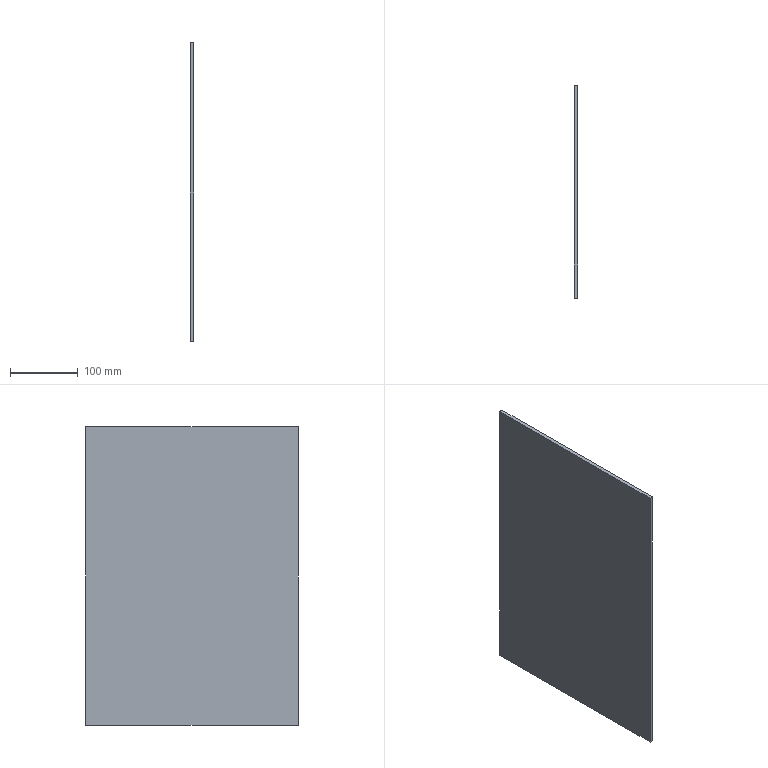Part | NX | features solid 2 | 1 solid | 6 faces | box 5 x 315 x 442 mm | volume 696150 mm3 | plane 6
STEP:
#1=CARTESIAN_POINT('',(2193.5,-894.,882.5));
#2=VERTEX_POINT('',#1);
#3=CARTESIAN_POINT('',(2193.5,-1209.,882.5));
#4=VERTEX_POINT('',#3);
#5=CARTESIAN_POINT('',(2193.5,-829.,882.5));
#6=DIRECTION('',(0.,-1.,0.));
#7=VECTOR('',#6,1000.);
#8=LINE('',#5,#7);
#9=EDGE_CURVE('',#2,#4,#8,.T.);
#10=ORIENTED_EDGE('',*,*,#9,.T.);
#11=CARTESIAN_POINT('',(2193.5,-1209.,440.5));
#12=VERTEX_POINT('',#11);
#13=CARTESIAN_POINT('',(2193.5,-1209.,972.5));
#14=DIRECTION('',(0.,0.,-1.));
#15=VECTOR('',#14,1000.);
#16=LINE('',#13,#15);
#17=EDGE_CURVE('',#4,#12,#16,.T.);
#18=ORIENTED_EDGE('',*,*,#17,.T.);
#19=CARTESIAN_POINT('',(2193.5,-894.,440.5));
#20=VERTEX_POINT('',#19);
#21=CARTESIAN_POINT('',(2193.5,-829.,440.5));
#22=DIRECTION('',(0.,1.,0.));
#23=VECTOR('',#22,1000.);
#24=LINE('',#21,#23);
#25=EDGE_CURVE('',#12,#20,#24,.T.);
#26=ORIENTED_EDGE('',*,*,#25,.T.);
#27=CARTESIAN_POINT('',(2193.5,-894.,972.5));
#28=DIRECTION('',(0.,0.,1.));
#29=VECTOR('',#28,1000.);
#30=LINE('',#27,#29);
#31=EDGE_CURVE('',#20,#2,#30,.T.);
#32=ORIENTED_EDGE('',*,*,#31,.T.);
#33=EDGE_LOOP('',(#10,#18,#26,#32));
#34=FACE_BOUND('',#33,.T.);
#35=CARTESIAN_POINT('',(2193.5,-829.,972.5));
#36=DIRECTION('',(1.,0.,0.));
#37=DIRECTION('',(0.,0.,-1.));
#38=AXIS2_PLACEMENT_3D('',#35,#36,#37);
#39=PLANE('',#38);
#40=ADVANCED_FACE('',(#34),#39,.T.);
#41=ORIENTED_EDGE('',*,*,#31,.F.);
#42=CARTESIAN_POINT('',(2188.5,-894.,440.5));
#43=VERTEX_POINT('',#42);
#44=CARTESIAN_POINT('',(2188.5,-894.,440.5));
#45=DIRECTION('',(-1.,0.,0.));
#46=VECTOR('',#45,1000.);
#47=LINE('',#44,#46);
#48=EDGE_CURVE('',#20,#43,#47,.T.);
#49=ORIENTED_EDGE('',*,*,#48,.T.);
#50=CARTESIAN_POINT('',(2188.5,-894.,882.5));
#51=VERTEX_POINT('',#50);
#52=CARTESIAN_POINT('',(2188.5,-894.,972.5));
#53=DIRECTION('',(0.,0.,1.));
#54=VECTOR('',#53,1000.);
#55=LINE('',#52,#54);
#56=EDGE_CURVE('',#43,#51,#55,.T.);
#57=ORIENTED_EDGE('',*,*,#56,.T.);
#58=CARTESIAN_POINT('',(2188.5,-894.,882.5));
#59=DIRECTION('',(-1.,0.,0.));
#60=VECTOR('',#59,1000.);
#61=LINE('',#58,#60);
#62=EDGE_CURVE('',#2,#51,#61,.T.);
#63=ORIENTED_EDGE('',*,*,#62,.F.);
#64=EDGE_LOOP('',(#41,#49,#57,#63));
#65=FACE_BOUND('',#64,.T.);
#66=CARTESIAN_POINT('',(2188.5,-894.,972.5));
#67=DIRECTION('',(0.,1.,0.));
#68=DIRECTION('',(0.,0.,-1.));
#69=AXIS2_PLACEMENT_3D('',#66,#67,#68);
#70=PLANE('',#69);
#71=ADVANCED_FACE('',(#65),#70,.T.);
#72=CARTESIAN_POINT('',(2188.5,-1209.,440.5));
#73=VERTEX_POINT('',#72);
#74=CARTESIAN_POINT('',(2188.5,-1209.,440.5));
#75=DIRECTION('',(-1.,0.,0.));
#76=VECTOR('',#75,1000.);
#77=LINE('',#74,#76);
#78=EDGE_CURVE('',#12,#73,#77,.T.);
#79=ORIENTED_EDGE('',*,*,#78,.T.);
#80=CARTESIAN_POINT('',(2188.5,-829.,440.5));
#81=DIRECTION('',(0.,1.,0.));
#82=VECTOR('',#81,1000.);
#83=LINE('',#80,#82);
#84=EDGE_CURVE('',#73,#43,#83,.T.);
#85=ORIENTED_EDGE('',*,*,#84,.T.);
#86=ORIENTED_EDGE('',*,*,#48,.F.);
#87=ORIENTED_EDGE('',*,*,#25,.F.);
#88=EDGE_LOOP('',(#79,#85,#86,#87));
#89=FACE_BOUND('',#88,.T.);
#90=CARTESIAN_POINT('',(2188.5,-829.,440.5));
#91=DIRECTION('',(0.,0.,-1.));
#92=DIRECTION('',(0.,-1.,0.));
#93=AXIS2_PLACEMENT_3D('',#90,#91,#92);
#94=PLANE('',#93);
#95=ADVANCED_FACE('',(#89),#94,.T.);
#96=CARTESIAN_POINT('',(2188.5,-1209.,882.5));
#97=VERTEX_POINT('',#96);
#98=CARTESIAN_POINT('',(2188.5,-1209.,882.5));
#99=DIRECTION('',(-1.,0.,0.));
#100=VECTOR('',#99,1000.);
#101=LINE('',#98,#100);
#102=EDGE_CURVE('',#4,#97,#101,.T.);
#103=ORIENTED_EDGE('',*,*,#102,.T.);
#104=CARTESIAN_POINT('',(2188.5,-1209.,972.5));
#105=DIRECTION('',(0.,0.,-1.));
#106=VECTOR('',#105,1000.);
#107=LINE('',#104,#106);
#108=EDGE_CURVE('',#97,#73,#107,.T.);
#109=ORIENTED_EDGE('',*,*,#108,.T.);
#110=ORIENTED_EDGE('',*,*,#78,.F.);
#111=ORIENTED_EDGE('',*,*,#17,.F.);
#112=EDGE_LOOP('',(#103,#109,#110,#111));
#113=FACE_BOUND('',#112,.T.);
#114=CARTESIAN_POINT('',(2188.5,-1209.,972.5));
#115=DIRECTION('',(0.,-1.,0.));
#116=DIRECTION('',(-1.,0.,0.));
#117=AXIS2_PLACEMENT_3D('',#114,#115,#116);
#118=PLANE('',#117);
#119=ADVANCED_FACE('',(#113),#118,.T.);
#120=ORIENTED_EDGE('',*,*,#62,.T.);
#121=CARTESIAN_POINT('',(2188.5,-829.,882.5));
#122=DIRECTION('',(0.,-1.,0.));
#123=VECTOR('',#122,1000.);
#124=LINE('',#121,#123);
#125=EDGE_CURVE('',#51,#97,#124,.T.);
#126=ORIENTED_EDGE('',*,*,#125,.T.);
#127=ORIENTED_EDGE('',*,*,#102,.F.);
#128=ORIENTED_EDGE('',*,*,#9,.F.);
#129=EDGE_LOOP('',(#120,#126,#127,#128));
#130=FACE_BOUND('',#129,.T.);
#131=CARTESIAN_POINT('',(2188.5,-829.,882.5));
#132=DIRECTION('',(0.,0.,1.));
#133=DIRECTION('',(0.,-1.,0.));
#134=AXIS2_PLACEMENT_3D('',#131,#132,#133);
#135=PLANE('',#134);
#136=ADVANCED_FACE('',(#130),#135,.T.);
#137=ORIENTED_EDGE('',*,*,#108,.F.);
#138=ORIENTED_EDGE('',*,*,#125,.F.);
#139=ORIENTED_EDGE('',*,*,#56,.F.);
#140=ORIENTED_EDGE('',*,*,#84,.F.);
#141=EDGE_LOOP('',(#137,#138,#139,#140));
#142=FACE_BOUND('',#141,.T.);
#143=CARTESIAN_POINT('',(2188.5,-829.,972.5));
#144=DIRECTION('',(1.,0.,0.));
#145=DIRECTION('',(0.,0.,-1.));
#146=AXIS2_PLACEMENT_3D('',#143,#144,#145);
#147=PLANE('',#146);
#148=ADVANCED_FACE('',(#142),#147,.F.);
#149=CLOSED_SHELL('',(#40,#71,#95,#119,#136,#148));
#150=MANIFOLD_SOLID_BREP('',#149);
#151=(LENGTH_UNIT()NAMED_UNIT(*)SI_UNIT(.MILLI.,.METRE.));
#152=UNCERTAINTY_MEASURE_WITH_UNIT(LENGTH_MEASURE(0.00001),#151,'','');
#153=(NAMED_UNIT(*)PLANE_ANGLE_UNIT()SI_UNIT($,.RADIAN.));
#154=(NAMED_UNIT(*)SI_UNIT($,.STERADIAN.)SOLID_ANGLE_UNIT());
#155=(GEOMETRIC_REPRESENTATION_CONTEXT(3)GLOBAL_UNCERTAINTY_ASSIGNED_CONTEXT((#152))GLOBAL_UNIT_ASSIGNED_CONTEXT((#151,#153,#154))REPRESENTATION_CONTEXT('',''));
#156=ADVANCED_BREP_SHAPE_REPRESENTATION('',(#150),#155);